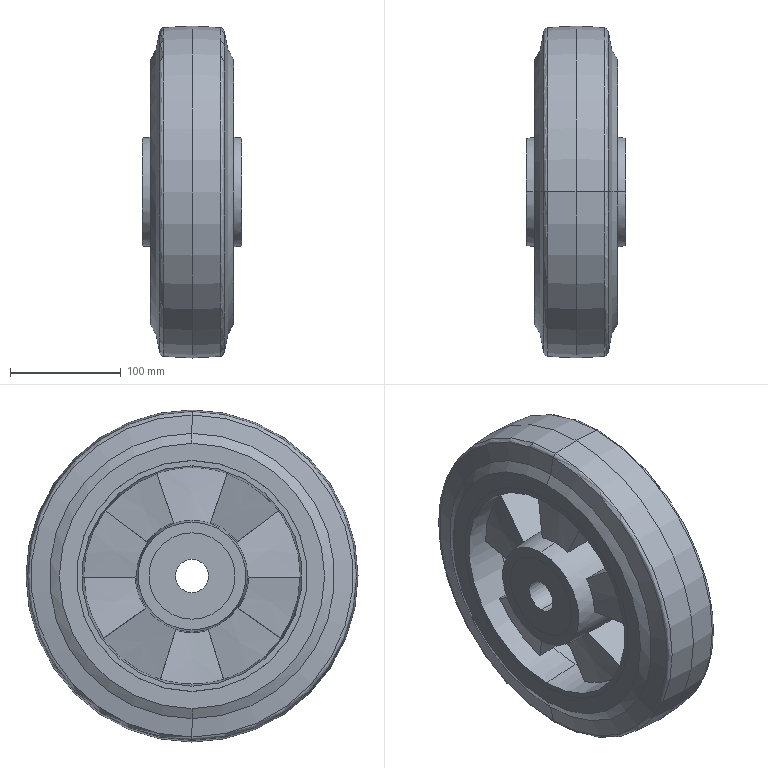Part | SolidWorks | features BaseBody 1, Scale 1 | 1 solid | 100 faces | box 90 x 300 x 300 mm | volume 3470694 mm3 | cone 32 | plane 30 | torus 24 | cylinder 14 | commonest cylinder face diameters 78 x4 208.618 x4 208.768 x4 30 x2